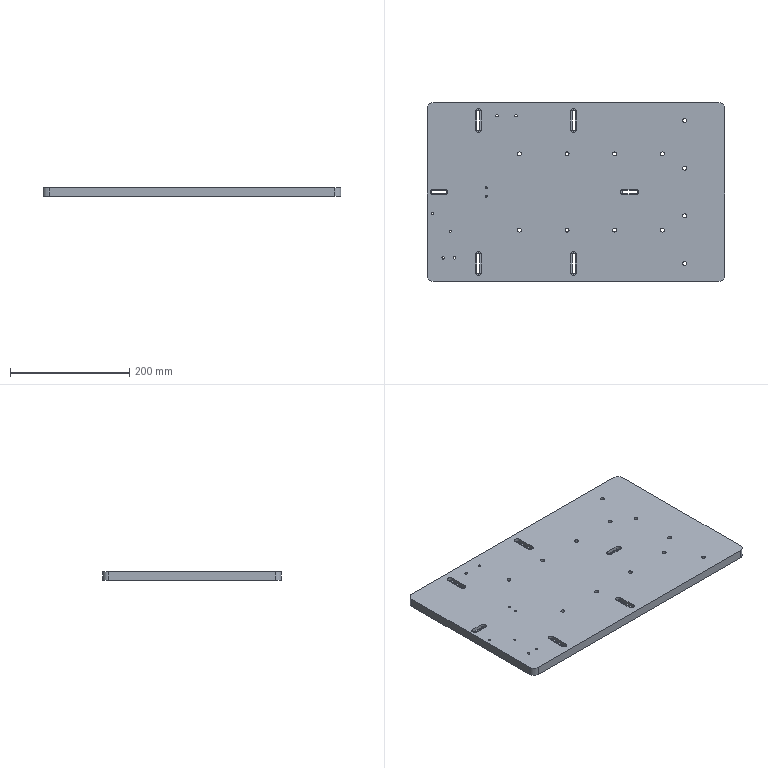Part | STEP file | KF-2212-060-001 | 1 solid | 144 faces | box 500 x 300 x 15 mm | volume 2214931 mm3 | cylinder 96 | plane 48 | commonest cylinder face diameters 6.6 x24 11 x24 5.5 x14 10 x14 3.3 x8 4.2 x8